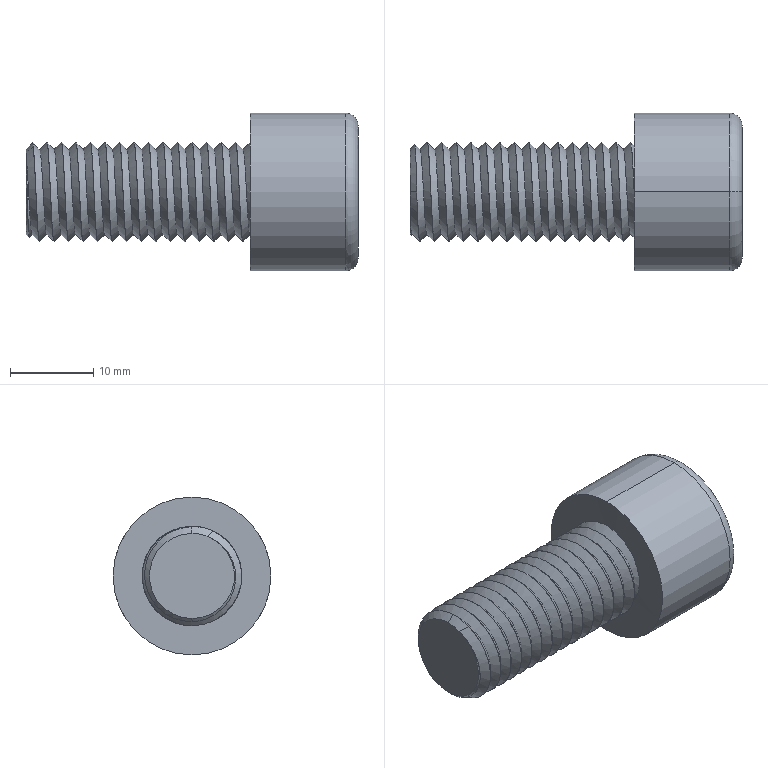Part | SolidWorks | features BaseBody 1 | 1 solid | 49 faces | box 40 x 19 x 19 mm | volume 5409 mm3 | cylinder 32 | plane 10 | cone 3 | spline 2 | torus 2 | commonest cylinder face diameters 12 x30 19 x2